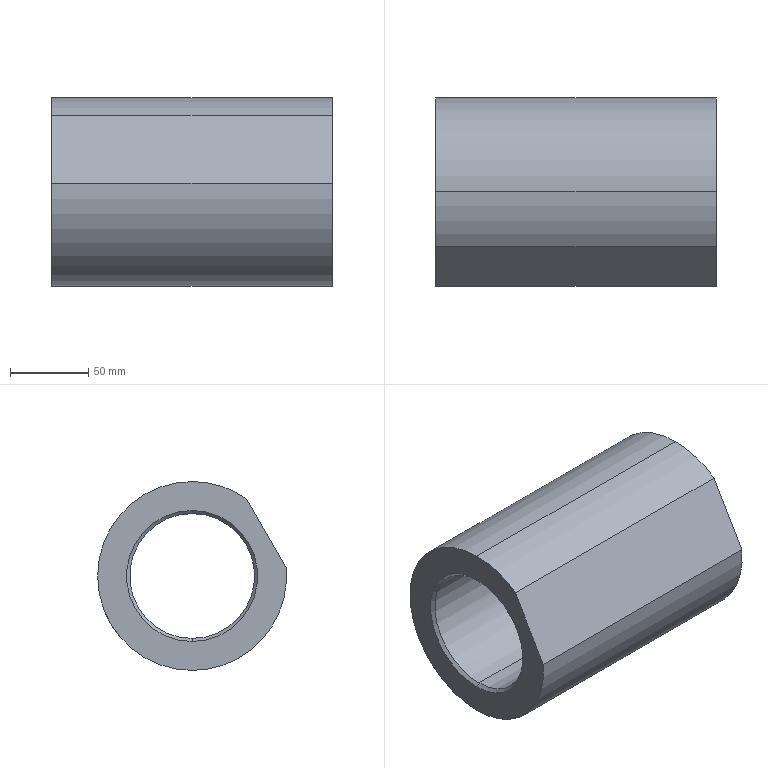Part | SolidWorks | features HoleWzd 2, Chamfer 1, Extrusion 1, ICE 1 | 1 solid | 30 faces | box 180 x 121 x 121 mm | volume 1121817 mm3 | cylinder 15 | cone 12 | plane 3 | commonest cylinder face diameters 8.5 x10 121 x3 80 x2
STEP:
#1=CARTESIAN_POINT('',(88.,0.,40.));
#2=VERTEX_POINT('',#1);
#3=CARTESIAN_POINT('',(88.,0.,-40.));
#4=VERTEX_POINT('',#3);
#5=CARTESIAN_POINT('',(88.,0.,0.));
#6=DIRECTION('',(1.,0.,0.));
#7=DIRECTION('',(0.,0.,-1.));
#8=AXIS2_PLACEMENT_3D('',#5,#6,#7);
#9=CIRCLE('',#8,40.);
#10=EDGE_CURVE('',#2,#4,#9,.T.);
#11=ORIENTED_EDGE('',*,*,#10,.F.);
#12=CARTESIAN_POINT('',(90.,0.,42.));
#13=VERTEX_POINT('',#12);
#14=CARTESIAN_POINT('',(88.,0.,40.));
#15=DIRECTION('',(0.7071,0.,0.7071));
#16=VECTOR('',#15,1000.);
#17=LINE('',#14,#16);
#18=EDGE_CURVE('',#2,#13,#17,.T.);
#19=ORIENTED_EDGE('',*,*,#18,.T.);
#20=CARTESIAN_POINT('',(90.,0.,-42.));
#21=VERTEX_POINT('',#20);
#22=CARTESIAN_POINT('',(90.,0.,0.));
#23=DIRECTION('',(-1.,0.,0.));
#24=DIRECTION('',(0.,0.,-1.));
#25=AXIS2_PLACEMENT_3D('',#22,#23,#24);
#26=CIRCLE('',#25,42.);
#27=EDGE_CURVE('',#21,#13,#26,.T.);
#28=ORIENTED_EDGE('',*,*,#27,.F.);
#29=CARTESIAN_POINT('',(88.,0.,-40.));
#30=DIRECTION('',(0.7071,0.,-0.7071));
#31=VECTOR('',#30,1000.);
#32=LINE('',#29,#31);
#33=EDGE_CURVE('',#4,#21,#32,.T.);
#34=ORIENTED_EDGE('',*,*,#33,.F.);
#35=EDGE_LOOP('',(#11,#19,#28,#34));
#36=FACE_OUTER_BOUND('',#35,.T.);
#37=CARTESIAN_POINT('',(88.,0.,0.));
#38=DIRECTION('',(1.,0.,0.));
#39=DIRECTION('',(0.,0.,-1.));
#40=AXIS2_PLACEMENT_3D('',#37,#38,#39);
#41=CONICAL_SURFACE('',#40,40.,0.7854);
#42=ADVANCED_FACE('',(#36),#41,.F.);
#43=CARTESIAN_POINT('',(-88.,0.,-40.));
#44=VERTEX_POINT('',#43);
#45=CARTESIAN_POINT('',(-88.,0.,40.));
#46=VERTEX_POINT('',#45);
#47=CARTESIAN_POINT('',(-88.,0.,0.));
#48=DIRECTION('',(-1.,0.,0.));
#49=DIRECTION('',(0.,0.,-1.));
#50=AXIS2_PLACEMENT_3D('',#47,#48,#49);
#51=CIRCLE('',#50,40.);
#52=EDGE_CURVE('',#44,#46,#51,.T.);
#53=ORIENTED_EDGE('',*,*,#52,.F.);
#54=CARTESIAN_POINT('',(-90.,0.,-42.));
#55=VERTEX_POINT('',#54);
#56=CARTESIAN_POINT('',(-90.,0.,-42.));
#57=DIRECTION('',(-0.7071,0.,-0.7071));
#58=VECTOR('',#57,1000.);
#59=LINE('',#56,#58);
#60=EDGE_CURVE('',#44,#55,#59,.T.);
#61=ORIENTED_EDGE('',*,*,#60,.T.);
#62=CARTESIAN_POINT('',(-90.,0.,42.));
#63=VERTEX_POINT('',#62);
#64=CARTESIAN_POINT('',(-90.,0.,0.));
#65=DIRECTION('',(1.,0.,0.));
#66=DIRECTION('',(0.,0.,-1.));
#67=AXIS2_PLACEMENT_3D('',#64,#65,#66);
#68=CIRCLE('',#67,42.);
#69=EDGE_CURVE('',#63,#55,#68,.T.);
#70=ORIENTED_EDGE('',*,*,#69,.F.);
#71=CARTESIAN_POINT('',(-90.,0.,42.));
#72=DIRECTION('',(-0.7071,0.,0.7071));
#73=VECTOR('',#72,1000.);
#74=LINE('',#71,#73);
#75=EDGE_CURVE('',#46,#63,#74,.T.);
#76=ORIENTED_EDGE('',*,*,#75,.F.);
#77=EDGE_LOOP('',(#53,#61,#70,#76));
#78=FACE_OUTER_BOUND('',#77,.T.);
#79=CARTESIAN_POINT('',(-90.,0.,0.));
#80=DIRECTION('',(-1.,0.,0.));
#81=DIRECTION('',(0.,0.,1.));
#82=AXIS2_PLACEMENT_3D('',#79,#80,#81);
#83=CONICAL_SURFACE('',#82,42.,0.7854);
#84=ADVANCED_FACE('',(#78),#83,.F.);
#85=CARTESIAN_POINT('',(58.,49.81,8.608));
#86=VERTEX_POINT('',#85);
#87=CARTESIAN_POINT('',(58.,49.81,0.1078));
#88=VERTEX_POINT('',#87);
#89=CARTESIAN_POINT('',(58.,49.81,4.358));
#90=DIRECTION('',(1.,0.,0.));
#91=DIRECTION('',(0.,0.,-1.));
#92=AXIS2_PLACEMENT_3D('',#89,#90,#91);
#93=CIRCLE('',#92,4.25);
#94=EDGE_CURVE('',#86,#88,#93,.T.);
#95=ORIENTED_EDGE('',*,*,#94,.F.);
#96=CARTESIAN_POINT('',(90.,49.81,8.608));
#97=VERTEX_POINT('',#96);
#98=CARTESIAN_POINT('',(90.,49.81,8.608));
#99=DIRECTION('',(1.,0.,0.));
#100=VECTOR('',#99,1000.);
#101=LINE('',#98,#100);
#102=EDGE_CURVE('',#86,#97,#101,.T.);
#103=ORIENTED_EDGE('',*,*,#102,.T.);
#104=CARTESIAN_POINT('',(90.,49.81,0.1078));
#105=VERTEX_POINT('',#104);
#106=CARTESIAN_POINT('',(90.,49.81,4.358));
#107=DIRECTION('',(1.,0.,0.));
#108=DIRECTION('',(0.,0.,-1.));
#109=AXIS2_PLACEMENT_3D('',#106,#107,#108);
#110=CIRCLE('',#109,4.25);
#111=EDGE_CURVE('',#97,#105,#110,.T.);
#112=ORIENTED_EDGE('',*,*,#111,.T.);
#113=CARTESIAN_POINT('',(90.,49.81,0.1078));
#114=DIRECTION('',(1.,0.,0.));
#115=VECTOR('',#114,1000.);
#116=LINE('',#113,#115);
#117=EDGE_CURVE('',#88,#105,#116,.T.);
#118=ORIENTED_EDGE('',*,*,#117,.F.);
#119=EDGE_LOOP('',(#95,#103,#112,#118));
#120=FACE_OUTER_BOUND('',#119,.T.);
#121=CARTESIAN_POINT('',(90.,49.81,4.358));
#122=DIRECTION('',(1.,0.,0.));
#123=DIRECTION('',(0.,0.,-1.));
#124=AXIS2_PLACEMENT_3D('',#121,#122,#123);
#125=CYLINDRICAL_SURFACE('',#124,4.25);
#126=ADVANCED_FACE('',(#120),#125,.F.);
#127=CARTESIAN_POINT('',(55.446,49.81,4.358));
#128=VERTEX_POINT('',#127);
#129=CARTESIAN_POINT('',(58.,49.81,0.1078));
#130=DIRECTION('',(0.515,0.,-0.8572));
#131=VECTOR('',#130,1000.);
#132=LINE('',#129,#131);
#133=EDGE_CURVE('',#128,#88,#132,.T.);
#134=ORIENTED_EDGE('',*,*,#133,.F.);
#135=CARTESIAN_POINT('',(58.,49.81,8.608));
#136=DIRECTION('',(0.515,0.,0.8572));
#137=VECTOR('',#136,1000.);
#138=LINE('',#135,#137);
#139=EDGE_CURVE('',#128,#86,#138,.T.);
#140=ORIENTED_EDGE('',*,*,#139,.T.);
#141=ORIENTED_EDGE('',*,*,#94,.T.);
#142=EDGE_LOOP('',(#134,#140,#141));
#143=FACE_OUTER_BOUND('',#142,.T.);
#144=CARTESIAN_POINT('',(58.,49.81,4.358));
#145=DIRECTION('',(1.,0.,0.));
#146=DIRECTION('',(0.,0.,-1.));
#147=AXIS2_PLACEMENT_3D('',#144,#145,#146);
#148=CONICAL_SURFACE('',#147,4.25,1.03);
#149=ADVANCED_FACE('',(#143),#148,.F.);
#150=CARTESIAN_POINT('',(58.,21.131,-41.065));
#151=VERTEX_POINT('',#150);
#152=CARTESIAN_POINT('',(58.,21.131,-49.565));
#153=VERTEX_POINT('',#152);
#154=CARTESIAN_POINT('',(58.,21.131,-45.315));
#155=DIRECTION('',(1.,0.,0.));
#156=DIRECTION('',(0.,0.,-1.));
#157=AXIS2_PLACEMENT_3D('',#154,#155,#156);
#158=CIRCLE('',#157,4.25);
#159=EDGE_CURVE('',#151,#153,#158,.T.);
#160=ORIENTED_EDGE('',*,*,#159,.F.);
#161=CARTESIAN_POINT('',(90.,21.131,-41.065));
#162=VERTEX_POINT('',#161);
#163=CARTESIAN_POINT('',(90.,21.131,-41.065));
#164=DIRECTION('',(1.,0.,0.));
#165=VECTOR('',#164,1000.);
#166=LINE('',#163,#165);
#167=EDGE_CURVE('',#151,#162,#166,.T.);
#168=ORIENTED_EDGE('',*,*,#167,.T.);
#169=CARTESIAN_POINT('',(90.,21.131,-49.565));
#170=VERTEX_POINT('',#169);
#171=CARTESIAN_POINT('',(90.,21.131,-45.315));
#172=DIRECTION('',(1.,0.,0.));
#173=DIRECTION('',(0.,0.,-1.));
#174=AXIS2_PLACEMENT_3D('',#171,#172,#173);
#175=CIRCLE('',#174,4.25);
#176=EDGE_CURVE('',#162,#170,#175,.T.);
#177=ORIENTED_EDGE('',*,*,#176,.T.);
#178=CARTESIAN_POINT('',(90.,21.131,-49.565));
#179=DIRECTION('',(1.,0.,0.));
#180=VECTOR('',#179,1000.);
#181=LINE('',#178,#180);
#182=EDGE_CURVE('',#153,#170,#181,.T.);
#183=ORIENTED_EDGE('',*,*,#182,.F.);
#184=EDGE_LOOP('',(#160,#168,#177,#183));
#185=FACE_OUTER_BOUND('',#184,.T.);
#186=CARTESIAN_POINT('',(90.,21.131,-45.315));
#187=DIRECTION('',(1.,0.,0.));
#188=DIRECTION('',(0.,0.,-1.));
#189=AXIS2_PLACEMENT_3D('',#186,#187,#188);
#190=CYLINDRICAL_SURFACE('',#189,4.25);
#191=ADVANCED_FACE('',(#185),#190,.F.);
#192=CARTESIAN_POINT('',(55.446,21.131,-45.315));
#193=VERTEX_POINT('',#192);
#194=CARTESIAN_POINT('',(58.,21.131,-49.565));
#195=DIRECTION('',(0.515,0.,-0.8572));
#196=VECTOR('',#195,1000.);
#197=LINE('',#194,#196);
#198=EDGE_CURVE('',#193,#153,#197,.T.);
#199=ORIENTED_EDGE('',*,*,#198,.F.);
#200=CARTESIAN_POINT('',(58.,21.131,-41.065));
#201=DIRECTION('',(0.515,0.,0.8572));
#202=VECTOR('',#201,1000.);
#203=LINE('',#200,#202);
#204=EDGE_CURVE('',#193,#151,#203,.T.);
#205=ORIENTED_EDGE('',*,*,#204,.T.);
#206=ORIENTED_EDGE('',*,*,#159,.T.);
#207=EDGE_LOOP('',(#199,#205,#206));
#208=FACE_OUTER_BOUND('',#207,.T.);
#209=CARTESIAN_POINT('',(58.,21.131,-45.315));
#210=DIRECTION('',(1.,0.,0.));
#211=DIRECTION('',(0.,0.,-1.));
#212=AXIS2_PLACEMENT_3D('',#209,#210,#211);
#213=CONICAL_SURFACE('',#212,4.25,1.03);
#214=ADVANCED_FACE('',(#208),#213,.F.);
#215=CARTESIAN_POINT('',(58.,-35.355,-31.105));
#216=VERTEX_POINT('',#215);
#217=CARTESIAN_POINT('',(58.,-35.355,-39.605));
#218=VERTEX_POINT('',#217);
#219=CARTESIAN_POINT('',(58.,-35.355,-35.355));
#220=DIRECTION('',(1.,0.,0.));
#221=DIRECTION('',(0.,0.,-1.));
#222=AXIS2_PLACEMENT_3D('',#219,#220,#221);
#223=CIRCLE('',#222,4.25);
#224=EDGE_CURVE('',#216,#218,#223,.T.);
#225=ORIENTED_EDGE('',*,*,#224,.F.);
#226=CARTESIAN_POINT('',(90.,-35.355,-31.105));
#227=VERTEX_POINT('',#226);
#228=CARTESIAN_POINT('',(90.,-35.355,-31.105));
#229=DIRECTION('',(1.,0.,0.));
#230=VECTOR('',#229,1000.);
#231=LINE('',#228,#230);
#232=EDGE_CURVE('',#216,#227,#231,.T.);
#233=ORIENTED_EDGE('',*,*,#232,.T.);
#234=CARTESIAN_POINT('',(90.,-35.355,-39.605));
#235=VERTEX_POINT('',#234);
#236=CARTESIAN_POINT('',(90.,-35.355,-35.355));
#237=DIRECTION('',(1.,0.,0.));
#238=DIRECTION('',(0.,0.,-1.));
#239=AXIS2_PLACEMENT_3D('',#236,#237,#238);
#240=CIRCLE('',#239,4.25);
#241=EDGE_CURVE('',#227,#235,#240,.T.);
#242=ORIENTED_EDGE('',*,*,#241,.T.);
#243=CARTESIAN_POINT('',(90.,-35.355,-39.605));
#244=DIRECTION('',(1.,0.,0.));
#245=VECTOR('',#244,1000.);
#246=LINE('',#243,#245);
#247=EDGE_CURVE('',#218,#235,#246,.T.);
#248=ORIENTED_EDGE('',*,*,#247,.F.);
#249=EDGE_LOOP('',(#225,#233,#242,#248));
#250=FACE_OUTER_BOUND('',#249,.T.);
#251=CARTESIAN_POINT('',(90.,-35.355,-35.355));
#252=DIRECTION('',(1.,0.,0.));
#253=DIRECTION('',(0.,0.,-1.));
#254=AXIS2_PLACEMENT_3D('',#251,#252,#253);
#255=CYLINDRICAL_SURFACE('',#254,4.25);
#256=ADVANCED_FACE('',(#250),#255,.F.);
#257=CARTESIAN_POINT('',(55.446,-35.355,-35.355));
#258=VERTEX_POINT('',#257);
#259=CARTESIAN_POINT('',(58.,-35.355,-39.605));
#260=DIRECTION('',(0.515,0.,-0.8572));
#261=VECTOR('',#260,1000.);
#262=LINE('',#259,#261);
#263=EDGE_CURVE('',#258,#218,#262,.T.);
#264=ORIENTED_EDGE('',*,*,#263,.F.);
#265=CARTESIAN_POINT('',(58.,-35.355,-31.105));
#266=DIRECTION('',(0.515,0.,0.8572));
#267=VECTOR('',#266,1000.);
#268=LINE('',#265,#267);
#269=EDGE_CURVE('',#258,#216,#268,.T.);
#270=ORIENTED_EDGE('',*,*,#269,.T.);
#271=ORIENTED_EDGE('',*,*,#224,.T.);
#272=EDGE_LOOP('',(#264,#270,#271));
#273=FACE_OUTER_BOUND('',#272,.T.);
#274=CARTESIAN_POINT('',(58.,-35.355,-35.355));
#275=DIRECTION('',(1.,0.,0.));
#276=DIRECTION('',(0.,0.,-1.));
#277=AXIS2_PLACEMENT_3D('',#274,#275,#276);
#278=CONICAL_SURFACE('',#277,4.25,1.03);
#279=ADVANCED_FACE('',(#273),#278,.F.);
#280=CARTESIAN_POINT('',(58.,12.941,52.546));
#281=VERTEX_POINT('',#280);
#282=CARTESIAN_POINT('',(58.,12.941,44.046));
#283=VERTEX_POINT('',#282);
#284=CARTESIAN_POINT('',(58.,12.941,48.296));
#285=DIRECTION('',(1.,0.,0.));
#286=DIRECTION('',(0.,0.,-1.));
#287=AXIS2_PLACEMENT_3D('',#284,#285,#286);
#288=CIRCLE('',#287,4.25);
#289=EDGE_CURVE('',#281,#283,#288,.T.);
#290=ORIENTED_EDGE('',*,*,#289,.F.);
#291=CARTESIAN_POINT('',(90.,12.941,52.546));
#292=VERTEX_POINT('',#291);
#293=CARTESIAN_POINT('',(90.,12.941,52.546));
#294=DIRECTION('',(1.,0.,0.));
#295=VECTOR('',#294,1000.);
#296=LINE('',#293,#295);
#297=EDGE_CURVE('',#281,#292,#296,.T.);
#298=ORIENTED_EDGE('',*,*,#297,.T.);
#299=CARTESIAN_POINT('',(90.,12.941,44.046));
#300=VERTEX_POINT('',#299);
#301=CARTESIAN_POINT('',(90.,12.941,48.296));
#302=DIRECTION('',(1.,0.,0.));
#303=DIRECTION('',(0.,0.,-1.));
#304=AXIS2_PLACEMENT_3D('',#301,#302,#303);
#305=CIRCLE('',#304,4.25);
#306=EDGE_CURVE('',#292,#300,#305,.T.);
#307=ORIENTED_EDGE('',*,*,#306,.T.);
#308=CARTESIAN_POINT('',(90.,12.941,44.046));
#309=DIRECTION('',(1.,0.,0.));
#310=VECTOR('',#309,1000.);
#311=LINE('',#308,#310);
#312=EDGE_CURVE('',#283,#300,#311,.T.);
#313=ORIENTED_EDGE('',*,*,#312,.F.);
#314=EDGE_LOOP('',(#290,#298,#307,#313));
#315=FACE_OUTER_BOUND('',#314,.T.);
#316=CARTESIAN_POINT('',(90.,12.941,48.296));
#317=DIRECTION('',(1.,0.,0.));
#318=DIRECTION('',(0.,0.,-1.));
#319=AXIS2_PLACEMENT_3D('',#316,#317,#318);
#320=CYLINDRICAL_SURFACE('',#319,4.25);
#321=ADVANCED_FACE('',(#315),#320,.F.);
#322=CARTESIAN_POINT('',(55.446,12.941,48.296));
#323=VERTEX_POINT('',#322);
#324=CARTESIAN_POINT('',(58.,12.941,44.046));
#325=DIRECTION('',(0.515,0.,-0.8572));
#326=VECTOR('',#325,1000.);
#327=LINE('',#324,#326);
#328=EDGE_CURVE('',#323,#283,#327,.T.);
#329=ORIENTED_EDGE('',*,*,#328,.F.);
#330=CARTESIAN_POINT('',(58.,12.941,52.546));
#331=DIRECTION('',(0.515,0.,0.8572));
#332=VECTOR('',#331,1000.);
#333=LINE('',#330,#332);
#334=EDGE_CURVE('',#323,#281,#333,.T.);
#335=ORIENTED_EDGE('',*,*,#334,.T.);
#336=ORIENTED_EDGE('',*,*,#289,.T.);
#337=EDGE_LOOP('',(#329,#335,#336));
#338=FACE_OUTER_BOUND('',#337,.T.);
#339=CARTESIAN_POINT('',(58.,12.941,48.296));
#340=DIRECTION('',(1.,0.,0.));
#341=DIRECTION('',(0.,0.,-1.));
#342=AXIS2_PLACEMENT_3D('',#339,#340,#341);
#343=CONICAL_SURFACE('',#342,4.25,1.03);
#344=ADVANCED_FACE('',(#338),#343,.F.);
#345=CARTESIAN_POINT('',(0.,54.39,-26.495));
#346=VERTEX_POINT('',#345);
#347=CARTESIAN_POINT('',(0.,50.14,-33.856));
#348=VERTEX_POINT('',#347);
#349=CARTESIAN_POINT('',(0.,54.39,-26.495));
#350=CARTESIAN_POINT('',(-0.2774,54.39,-26.495));
#351=CARTESIAN_POINT('',(-0.5531,54.378,-26.519));
#352=CARTESIAN_POINT('',(-1.101,54.33,-26.617));
#353=CARTESIAN_POINT('',(-1.37,54.294,-26.69));
#354=CARTESIAN_POINT('',(-1.881,54.201,-26.881));
#355=CARTESIAN_POINT('',(-2.128,54.142,-26.999));
#356=CARTESIAN_POINT('',(-2.593,54.002,-27.277));
#357=CARTESIAN_POINT('',(-2.807,53.923,-27.434));
#358=CARTESIAN_POINT('',(-3.199,53.744,-27.783));
#359=CARTESIAN_POINT('',(-3.379,53.643,-27.977));
#360=CARTESIAN_POINT('',(-3.687,53.428,-28.386));
#361=CARTESIAN_POINT('',(-3.818,53.313,-28.601));
#362=CARTESIAN_POINT('',(-4.032,53.068,-29.053));
#363=CARTESIAN_POINT('',(-4.114,52.938,-29.29));
#364=CARTESIAN_POINT('',(-4.222,52.673,-29.764));
#365=CARTESIAN_POINT('',(-4.25,52.536,-30.004));
#366=CARTESIAN_POINT('',(-4.25,52.256,-30.49));
#367=CARTESIAN_POINT('',(-4.223,52.116,-30.729));
#368=CARTESIAN_POINT('',(-4.115,51.838,-31.196));
#369=CARTESIAN_POINT('',(-4.034,51.698,-31.426));
#370=CARTESIAN_POINT('',(-3.821,51.429,-31.866));
#371=CARTESIAN_POINT('',(-3.69,51.299,-32.073));
#372=CARTESIAN_POINT('',(-3.383,51.053,-32.464));
#373=CARTESIAN_POINT('',(-3.203,50.935,-32.648));
#374=CARTESIAN_POINT('',(-2.811,50.722,-32.978));
#375=CARTESIAN_POINT('',(-2.598,50.625,-33.126));
#376=CARTESIAN_POINT('',(-2.134,50.454,-33.386));
#377=CARTESIAN_POINT('',(-1.886,50.381,-33.497));
#378=CARTESIAN_POINT('',(-1.375,50.263,-33.674));
#379=CARTESIAN_POINT('',(-1.108,50.217,-33.742));
#380=CARTESIAN_POINT('',(-0.5587,50.156,-33.833));
#381=CARTESIAN_POINT('',(-0.2808,50.14,-33.856));
#382=CARTESIAN_POINT('',(0.,50.14,-33.856));
#383=B_SPLINE_CURVE_WITH_KNOTS('',3,(#349,#350,#351,#352,#353,#354,#355,#356,#357,#358,#359,#360,#361,#362,#363,#364,#365,#366,#367,#368,#369,#370,#371,#372,#373,#374,#375,#376,#377,#378,#379,#380,#381,#382),.UNSPECIFIED.,.F.,.F.,(4,2,2,2,2,2,2,2,2,2,2,2,2,2,2,2,4),(0.01329,0.01412,0.01495,0.01578,0.01661,0.01744,0.01827,0.01911,0.01994,0.02077,0.0216,0.02243,0.02326,0.02409,0.02492,0.02575,0.02658),.UNSPECIFIED.);
#384=EDGE_CURVE('',#346,#348,#383,.T.);
#385=ORIENTED_EDGE('',*,*,#384,.F.);
#386=CARTESIAN_POINT('',(0.,36.57,-16.206));
#387=VERTEX_POINT('',#386);
#388=CARTESIAN_POINT('',(0.,2.125,3.681));
#389=DIRECTION('',(0.,-0.866,0.5));
#390=VECTOR('',#389,1000.);
#391=LINE('',#388,#390);
#392=EDGE_CURVE('',#346,#387,#391,.T.);
#393=ORIENTED_EDGE('',*,*,#392,.T.);
#394=CARTESIAN_POINT('',(0.,32.32,-23.567));
#395=VERTEX_POINT('',#394);
#396=CARTESIAN_POINT('',(0.,36.57,-16.206));
#397=CARTESIAN_POINT('',(-0.2774,36.57,-16.206));
#398=CARTESIAN_POINT('',(-0.5533,36.559,-16.231));
#399=CARTESIAN_POINT('',(-1.102,36.514,-16.331));
#400=CARTESIAN_POINT('',(-1.37,36.481,-16.406));
#401=CARTESIAN_POINT('',(-1.881,36.393,-16.6));
#402=CARTESIAN_POINT('',(-2.129,36.338,-16.72));
#403=CARTESIAN_POINT('',(-2.593,36.207,-17.003));
#404=CARTESIAN_POINT('',(-2.807,36.132,-17.162));
#405=CARTESIAN_POINT('',(-3.199,35.962,-17.516));
#406=CARTESIAN_POINT('',(-3.379,35.865,-17.713));
#407=CARTESIAN_POINT('',(-3.687,35.658,-18.126));
#408=CARTESIAN_POINT('',(-3.818,35.547,-18.343));
#409=CARTESIAN_POINT('',(-4.032,35.308,-18.799));
#410=CARTESIAN_POINT('',(-4.114,35.18,-19.037));
#411=CARTESIAN_POINT('',(-4.222,34.919,-19.513));
#412=CARTESIAN_POINT('',(-4.25,34.783,-19.754));
#413=CARTESIAN_POINT('',(-4.25,34.502,-20.24));
#414=CARTESIAN_POINT('',(-4.223,34.361,-20.478));
#415=CARTESIAN_POINT('',(-4.115,34.08,-20.943));
#416=CARTESIAN_POINT('',(-4.034,33.938,-21.173));
#417=CARTESIAN_POINT('',(-3.821,33.662,-21.608));
#418=CARTESIAN_POINT('',(-3.69,33.529,-21.814));
#419=CARTESIAN_POINT('',(-3.382,33.275,-22.2));
#420=CARTESIAN_POINT('',(-3.203,33.152,-22.382));
#421=CARTESIAN_POINT('',(-2.812,32.931,-22.707));
#422=CARTESIAN_POINT('',(-2.598,32.83,-22.852));
#423=CARTESIAN_POINT('',(-2.134,32.651,-23.107));
#424=CARTESIAN_POINT('',(-1.887,32.574,-23.215));
#425=CARTESIAN_POINT('',(-1.376,32.449,-23.389));
#426=CARTESIAN_POINT('',(-1.108,32.401,-23.456));
#427=CARTESIAN_POINT('',(-0.5588,32.336,-23.545));
#428=CARTESIAN_POINT('',(-0.281,32.32,-23.567));
#429=CARTESIAN_POINT('',(0.,32.32,-23.567));
#430=B_SPLINE_CURVE_WITH_KNOTS('',3,(#396,#397,#398,#399,#400,#401,#402,#403,#404,#405,#406,#407,#408,#409,#410,#411,#412,#413,#414,#415,#416,#417,#418,#419,#420,#421,#422,#423,#424,#425,#426,#427,#428,#429),.UNSPECIFIED.,.F.,.F.,(4,2,2,2,2,2,2,2,2,2,2,2,2,2,2,2,4),(0.0133,0.01413,0.01496,0.01579,0.01662,0.01745,0.01828,0.01911,0.01994,0.02077,0.02161,0.02244,0.02327,0.0241,0.02493,0.02576,0.02659),.UNSPECIFIED.);
#431=EDGE_CURVE('',#387,#395,#430,.T.);
#432=ORIENTED_EDGE('',*,*,#431,.T.);
#433=CARTESIAN_POINT('',(0.,-2.125,-3.681));
#434=DIRECTION('',(0.,-0.866,0.5));
#435=VECTOR('',#434,1000.);
#436=LINE('',#433,#435);
#437=EDGE_CURVE('',#348,#395,#436,.T.);
#438=ORIENTED_EDGE('',*,*,#437,.F.);
#439=EDGE_LOOP('',(#385,#393,#432,#438));
#440=FACE_OUTER_BOUND('',#439,.T.);
#441=CARTESIAN_POINT('',(0.,0.,0.));
#442=DIRECTION('',(0.,-0.866,0.5));
#443=DIRECTION('',(0.,-0.5,-0.866));
#444=AXIS2_PLACEMENT_3D('',#441,#442,#443);
#445=CYLINDRICAL_SURFACE('',#444,4.25);
#446=ADVANCED_FACE('',(#440),#445,.F.);
#447=ORIENTED_EDGE('',*,*,#10,.T.);
#448=CARTESIAN_POINT('',(90.,0.,-40.));
#449=DIRECTION('',(-1.,0.,0.));
#450=VECTOR('',#449,1000.);
#451=LINE('',#448,#450);
#452=EDGE_CURVE('',#4,#44,#451,.T.);
#453=ORIENTED_EDGE('',*,*,#452,.T.);
#454=ORIENTED_EDGE('',*,*,#52,.T.);
#455=CARTESIAN_POINT('',(90.,0.,40.));
#456=DIRECTION('',(-1.,0.,0.));
#457=VECTOR('',#456,1000.);
#458=LINE('',#455,#457);
#459=EDGE_CURVE('',#2,#46,#458,.T.);
#460=ORIENTED_EDGE('',*,*,#459,.F.);
#461=EDGE_LOOP('',(#447,#453,#454,#460));
#462=FACE_OUTER_BOUND('',#461,.T.);
#463=CARTESIAN_POINT('',(90.,0.,0.));
#464=DIRECTION('',(-1.,0.,0.));
#465=DIRECTION('',(0.,0.,1.));
#466=AXIS2_PLACEMENT_3D('',#463,#464,#465);
#467=CYLINDRICAL_SURFACE('',#466,40.);
#468=ADVANCED_FACE('',(#462),#467,.F.);
#469=CARTESIAN_POINT('',(0.,50.14,-33.856));
#470=CARTESIAN_POINT('',(0.2809,50.14,-33.856));
#471=CARTESIAN_POINT('',(0.5571,50.156,-33.833));
#472=CARTESIAN_POINT('',(1.1,50.216,-33.743));
#473=CARTESIAN_POINT('',(1.37,50.262,-33.675));
#474=CARTESIAN_POINT('',(1.885,50.381,-33.497));
#475=CARTESIAN_POINT('',(2.129,50.453,-33.388));
#476=CARTESIAN_POINT('',(2.591,50.623,-33.13));
#477=CARTESIAN_POINT('',(2.81,50.721,-32.98));
#478=CARTESIAN_POINT('',(3.202,50.934,-32.65));
#479=CARTESIAN_POINT('',(3.378,51.049,-32.469));
#480=CARTESIAN_POINT('',(3.688,51.297,-32.076));
#481=CARTESIAN_POINT('',(3.82,51.428,-31.866));
#482=CARTESIAN_POINT('',(4.032,51.696,-31.43));
#483=CARTESIAN_POINT('',(4.114,51.835,-31.201));
#484=CARTESIAN_POINT('',(4.223,52.116,-30.729));
#485=CARTESIAN_POINT('',(4.25,52.255,-30.491));
#486=CARTESIAN_POINT('',(4.25,52.532,-30.011));
#487=CARTESIAN_POINT('',(4.222,52.672,-29.766));
#488=CARTESIAN_POINT('',(4.114,52.938,-29.29));
#489=CARTESIAN_POINT('',(4.034,53.065,-29.058));
#490=CARTESIAN_POINT('',(3.821,53.311,-28.606));
#491=CARTESIAN_POINT('',(3.688,53.428,-28.386));
#492=CARTESIAN_POINT('',(3.38,53.643,-27.978));
#493=CARTESIAN_POINT('',(3.204,53.742,-27.787));
#494=CARTESIAN_POINT('',(2.807,53.923,-27.434));
#495=CARTESIAN_POINT('',(2.593,54.002,-27.277));
#496=CARTESIAN_POINT('',(2.132,54.141,-27.001));
#497=CARTESIAN_POINT('',(1.884,54.2,-26.882));
#498=CARTESIAN_POINT('',(1.369,54.295,-26.69));
#499=CARTESIAN_POINT('',(1.104,54.33,-26.618));
#500=CARTESIAN_POINT('',(0.5592,54.378,-26.52));
#501=CARTESIAN_POINT('',(0.2774,54.39,-26.495));
#502=CARTESIAN_POINT('',(0.,54.39,-26.495));
#503=B_SPLINE_CURVE_WITH_KNOTS('',3,(#469,#470,#471,#472,#473,#474,#475,#476,#477,#478,#479,#480,#481,#482,#483,#484,#485,#486,#487,#488,#489,#490,#491,#492,#493,#494,#495,#496,#497,#498,#499,#500,#501,#502),.UNSPECIFIED.,.F.,.F.,(4,2,2,2,2,2,2,2,2,2,2,2,2,2,2,2,4),(0.,0.0008307,0.001661,0.002492,0.003323,0.004154,0.004984,0.005815,0.006646,0.007476,0.008307,0.009138,0.009969,0.0108,0.01163,0.01246,0.01329),.UNSPECIFIED.);
#504=EDGE_CURVE('',#348,#346,#503,.T.);
#505=ORIENTED_EDGE('',*,*,#504,.T.);
#506=ORIENTED_EDGE('',*,*,#384,.T.);
#507=EDGE_LOOP('',(#505,#506));
#508=FACE_BOUND('',#507,.T.);
#509=CARTESIAN_POINT('',(90.,0.,-60.5));
#510=VERTEX_POINT('',#509);
#511=CARTESIAN_POINT('',(90.,0.,60.5));
#512=VERTEX_POINT('',#511);
#513=CARTESIAN_POINT('',(90.,0.,0.));
#514=DIRECTION('',(1.,0.,0.));
#515=DIRECTION('',(0.,0.,-1.));
#516=AXIS2_PLACEMENT_3D('',#513,#514,#515);
#517=CIRCLE('',#516,60.5);
#518=EDGE_CURVE('',#510,#512,#517,.T.);
#519=ORIENTED_EDGE('',*,*,#518,.F.);
#520=CARTESIAN_POINT('',(-90.,0.,-60.5));
#521=VERTEX_POINT('',#520);
#522=CARTESIAN_POINT('',(90.,0.,-60.5));
#523=DIRECTION('',(-1.,0.,0.));
#524=VECTOR('',#523,1000.);
#525=LINE('',#522,#524);
#526=EDGE_CURVE('',#510,#521,#525,.T.);
#527=ORIENTED_EDGE('',*,*,#526,.T.);
#528=CARTESIAN_POINT('',(-90.,0.,60.5));
#529=VERTEX_POINT('',#528);
#530=CARTESIAN_POINT('',(-90.,0.,0.));
#531=DIRECTION('',(1.,0.,0.));
#532=DIRECTION('',(0.,0.,-1.));
#533=AXIS2_PLACEMENT_3D('',#530,#531,#532);
#534=CIRCLE('',#533,60.5);
#535=EDGE_CURVE('',#521,#529,#534,.T.);
#536=ORIENTED_EDGE('',*,*,#535,.T.);
#537=CARTESIAN_POINT('',(90.,0.,60.5));
#538=DIRECTION('',(-1.,0.,0.));
#539=VECTOR('',#538,1000.);
#540=LINE('',#537,#539);
#541=EDGE_CURVE('',#512,#529,#540,.T.);
#542=ORIENTED_EDGE('',*,*,#541,.F.);
#543=EDGE_LOOP('',(#519,#527,#536,#542));
#544=FACE_OUTER_BOUND('',#543,.T.);
#545=CARTESIAN_POINT('',(90.,0.,0.));
#546=DIRECTION('',(-1.,0.,0.));
#547=DIRECTION('',(0.,0.,1.));
#548=AXIS2_PLACEMENT_3D('',#545,#546,#547);
#549=CYLINDRICAL_SURFACE('',#548,60.5);
#550=ADVANCED_FACE('',(#508,#544),#549,.T.);
#551=CARTESIAN_POINT('',(90.,-35.029,49.327));
#552=VERTEX_POINT('',#551);
#553=CARTESIAN_POINT('',(90.,0.,0.));
#554=DIRECTION('',(1.,0.,0.));
#555=DIRECTION('',(0.,0.,-1.));
#556=AXIS2_PLACEMENT_3D('',#553,#554,#555);
#557=CIRCLE('',#556,60.5);
#558=EDGE_CURVE('',#512,#552,#557,.T.);
#559=ORIENTED_EDGE('',*,*,#558,.F.);
#560=ORIENTED_EDGE('',*,*,#541,.T.);
#561=CARTESIAN_POINT('',(-90.,-35.029,49.327));
#562=VERTEX_POINT('',#561);
#563=CARTESIAN_POINT('',(-90.,0.,0.));
#564=DIRECTION('',(1.,0.,0.));
#565=DIRECTION('',(0.,0.,-1.));
#566=AXIS2_PLACEMENT_3D('',#563,#564,#565);
#567=CIRCLE('',#566,60.5);
#568=EDGE_CURVE('',#529,#562,#567,.T.);
#569=ORIENTED_EDGE('',*,*,#568,.T.);
#570=CARTESIAN_POINT('',(-90.,-35.029,49.327));
#571=DIRECTION('',(1.,0.,0.));
#572=VECTOR('',#571,1000.);
#573=LINE('',#570,#572);
#574=EDGE_CURVE('',#562,#552,#573,.T.);
#575=ORIENTED_EDGE('',*,*,#574,.T.);
#576=EDGE_LOOP('',(#559,#560,#569,#575));
#577=FACE_OUTER_BOUND('',#576,.T.);
#578=CARTESIAN_POINT('',(90.,0.,0.));
#579=DIRECTION('',(-1.,0.,0.));
#580=DIRECTION('',(0.,0.,1.));
#581=AXIS2_PLACEMENT_3D('',#578,#579,#580);
#582=CYLINDRICAL_SURFACE('',#581,60.5);
#583=ADVANCED_FACE('',(#577),#582,.T.);
#584=ORIENTED_EDGE('',*,*,#27,.T.);
#585=CARTESIAN_POINT('',(90.,0.,0.));
#586=DIRECTION('',(-1.,0.,0.));
#587=DIRECTION('',(0.,0.,-1.));
#588=AXIS2_PLACEMENT_3D('',#585,#586,#587);
#589=CIRCLE('',#588,42.);
#590=EDGE_CURVE('',#13,#21,#589,.T.);
#591=ORIENTED_EDGE('',*,*,#590,.T.);
#592=EDGE_LOOP('',(#584,#591));
#593=FACE_BOUND('',#592,.T.);
#594=CARTESIAN_POINT('',(90.,49.81,4.358));
#595=DIRECTION('',(1.,0.,0.));
#596=DIRECTION('',(0.,0.,-1.));
#597=AXIS2_PLACEMENT_3D('',#594,#595,#596);
#598=CIRCLE('',#597,4.25);
#599=EDGE_CURVE('',#105,#97,#598,.T.);
#600=ORIENTED_EDGE('',*,*,#599,.F.);
#601=ORIENTED_EDGE('',*,*,#111,.F.);
#602=EDGE_LOOP('',(#600,#601));
#603=FACE_BOUND('',#602,.T.);
#604=CARTESIAN_POINT('',(90.,21.131,-45.315));
#605=DIRECTION('',(1.,0.,0.));
#606=DIRECTION('',(0.,0.,-1.));
#607=AXIS2_PLACEMENT_3D('',#604,#605,#606);
#608=CIRCLE('',#607,4.25);
#609=EDGE_CURVE('',#170,#162,#608,.T.);
#610=ORIENTED_EDGE('',*,*,#609,.F.);
#611=ORIENTED_EDGE('',*,*,#176,.F.);
#612=EDGE_LOOP('',(#610,#611));
#613=FACE_BOUND('',#612,.T.);
#614=CARTESIAN_POINT('',(90.,-35.355,-35.355));
#615=DIRECTION('',(1.,0.,0.));
#616=DIRECTION('',(0.,0.,-1.));
#617=AXIS2_PLACEMENT_3D('',#614,#615,#616);
#618=CIRCLE('',#617,4.25);
#619=EDGE_CURVE('',#235,#227,#618,.T.);
#620=ORIENTED_EDGE('',*,*,#619,.F.);
#621=ORIENTED_EDGE('',*,*,#241,.F.);
#622=EDGE_LOOP('',(#620,#621));
#623=FACE_BOUND('',#622,.T.);
#624=CARTESIAN_POINT('',(90.,12.941,48.296));
#625=DIRECTION('',(1.,0.,0.));
#626=DIRECTION('',(0.,0.,-1.));
#627=AXIS2_PLACEMENT_3D('',#624,#625,#626);
#628=CIRCLE('',#627,4.25);
#629=EDGE_CURVE('',#300,#292,#628,.T.);
#630=ORIENTED_EDGE('',*,*,#629,.F.);
#631=ORIENTED_EDGE('',*,*,#306,.F.);
#632=EDGE_LOOP('',(#630,#631));
#633=FACE_BOUND('',#632,.T.);
#634=CARTESIAN_POINT('',(90.,-60.233,5.673));
#635=VERTEX_POINT('',#634);
#636=CARTESIAN_POINT('',(90.,-35.029,49.327));
#637=DIRECTION('',(0.,0.5,0.866));
#638=VECTOR('',#637,1000.);
#639=LINE('',#636,#638);
#640=EDGE_CURVE('',#635,#552,#639,.T.);
#641=ORIENTED_EDGE('',*,*,#640,.F.);
#642=CARTESIAN_POINT('',(90.,0.,0.));
#643=DIRECTION('',(1.,0.,0.));
#644=DIRECTION('',(0.,0.,-1.));
#645=AXIS2_PLACEMENT_3D('',#642,#643,#644);
#646=CIRCLE('',#645,60.5);
#647=EDGE_CURVE('',#635,#510,#646,.T.);
#648=ORIENTED_EDGE('',*,*,#647,.T.);
#649=ORIENTED_EDGE('',*,*,#518,.T.);
#650=ORIENTED_EDGE('',*,*,#558,.T.);
#651=EDGE_LOOP('',(#641,#648,#649,#650));
#652=FACE_OUTER_BOUND('',#651,.T.);
#653=CARTESIAN_POINT('',(90.,0.,0.));
#654=DIRECTION('',(1.,0.,0.));
#655=DIRECTION('',(0.,0.,-1.));
#656=AXIS2_PLACEMENT_3D('',#653,#654,#655);
#657=PLANE('',#656);
#658=ADVANCED_FACE('',(#593,#603,#613,#623,#633,#652),#657,.T.);
#659=ORIENTED_EDGE('',*,*,#69,.T.);
#660=CARTESIAN_POINT('',(-90.,0.,0.));
#661=DIRECTION('',(1.,0.,0.));
#662=DIRECTION('',(0.,0.,-1.));
#663=AXIS2_PLACEMENT_3D('',#660,#661,#662);
#664=CIRCLE('',#663,42.);
#665=EDGE_CURVE('',#55,#63,#664,.T.);
#666=ORIENTED_EDGE('',*,*,#665,.T.);
#667=EDGE_LOOP('',(#659,#666));
#668=FACE_BOUND('',#667,.T.);
#669=CARTESIAN_POINT('',(-90.,-60.233,5.673));
#670=VERTEX_POINT('',#669);
#671=CARTESIAN_POINT('',(-90.,0.,0.));
#672=DIRECTION('',(1.,0.,0.));
#673=DIRECTION('',(0.,0.,-1.));
#674=AXIS2_PLACEMENT_3D('',#671,#672,#673);
#675=CIRCLE('',#674,60.5);
#676=EDGE_CURVE('',#670,#521,#675,.T.);
#677=ORIENTED_EDGE('',*,*,#676,.F.);
#678=CARTESIAN_POINT('',(-90.,-35.029,49.327));
#679=DIRECTION('',(0.,0.5,0.866));
#680=VECTOR('',#679,1000.);
#681=LINE('',#678,#680);
#682=EDGE_CURVE('',#670,#562,#681,.T.);
#683=ORIENTED_EDGE('',*,*,#682,.T.);
#684=ORIENTED_EDGE('',*,*,#568,.F.);
#685=ORIENTED_EDGE('',*,*,#535,.F.);
#686=EDGE_LOOP('',(#677,#683,#684,#685));
#687=FACE_OUTER_BOUND('',#686,.T.);
#688=CARTESIAN_POINT('',(-90.,0.,0.));
#689=DIRECTION('',(1.,0.,0.));
#690=DIRECTION('',(0.,0.,-1.));
#691=AXIS2_PLACEMENT_3D('',#688,#689,#690);
#692=PLANE('',#691);
#693=ADVANCED_FACE('',(#668,#687),#692,.F.);
#694=ORIENTED_EDGE('',*,*,#526,.F.);
#695=ORIENTED_EDGE('',*,*,#647,.F.);
#696=CARTESIAN_POINT('',(-90.,-60.233,5.673));
#697=DIRECTION('',(1.,0.,0.));
#698=VECTOR('',#697,1000.);
#699=LINE('',#696,#698);
#700=EDGE_CURVE('',#670,#635,#699,.T.);
#701=ORIENTED_EDGE('',*,*,#700,.F.);
#702=ORIENTED_EDGE('',*,*,#676,.T.);
#703=EDGE_LOOP('',(#694,#695,#701,#702));
#704=FACE_OUTER_BOUND('',#703,.T.);
#705=CARTESIAN_POINT('',(90.,0.,0.));
#706=DIRECTION('',(-1.,0.,0.));
#707=DIRECTION('',(0.,0.,1.));
#708=AXIS2_PLACEMENT_3D('',#705,#706,#707);
#709=CYLINDRICAL_SURFACE('',#708,60.5);
#710=ADVANCED_FACE('',(#704),#709,.T.);
#711=ORIENTED_EDGE('',*,*,#452,.F.);
#712=CARTESIAN_POINT('',(88.,0.,0.));
#713=DIRECTION('',(1.,0.,0.));
#714=DIRECTION('',(0.,0.,-1.));
#715=AXIS2_PLACEMENT_3D('',#712,#713,#714);
#716=CIRCLE('',#715,40.);
#717=EDGE_CURVE('',#4,#2,#716,.T.);
#718=ORIENTED_EDGE('',*,*,#717,.T.);
#719=ORIENTED_EDGE('',*,*,#459,.T.);
#720=CARTESIAN_POINT('',(-88.,0.,0.));
#721=DIRECTION('',(-1.,0.,0.));
#722=DIRECTION('',(0.,0.,-1.));
#723=AXIS2_PLACEMENT_3D('',#720,#721,#722);
#724=CIRCLE('',#723,40.);
#725=EDGE_CURVE('',#46,#44,#724,.T.);
#726=ORIENTED_EDGE('',*,*,#725,.T.);
#727=EDGE_LOOP('',(#711,#718,#719,#726));
#728=FACE_OUTER_BOUND('',#727,.T.);
#729=CARTESIAN_POINT('',(0.,32.32,-23.567));
#730=CARTESIAN_POINT('',(0.281,32.32,-23.567));
#731=CARTESIAN_POINT('',(0.5573,32.336,-23.545));
#732=CARTESIAN_POINT('',(1.101,32.4,-23.457));
#733=CARTESIAN_POINT('',(1.371,32.448,-23.39));
#734=CARTESIAN_POINT('',(1.885,32.573,-23.216));
#735=CARTESIAN_POINT('',(2.13,32.649,-23.109));
#736=CARTESIAN_POINT('',(2.591,32.827,-22.856));
#737=CARTESIAN_POINT('',(2.81,32.93,-22.708));
#738=CARTESIAN_POINT('',(3.202,33.152,-22.383));
#739=CARTESIAN_POINT('',(3.378,33.271,-22.205));
#740=CARTESIAN_POINT('',(3.688,33.527,-21.817));
#741=CARTESIAN_POINT('',(3.82,33.662,-21.609));
#742=CARTESIAN_POINT('',(4.032,33.935,-21.177));
#743=CARTESIAN_POINT('',(4.114,34.077,-20.949));
#744=CARTESIAN_POINT('',(4.223,34.361,-20.479));
#745=CARTESIAN_POINT('',(4.25,34.502,-20.242));
#746=CARTESIAN_POINT('',(4.25,34.779,-19.761));
#747=CARTESIAN_POINT('',(4.222,34.917,-19.516));
#748=CARTESIAN_POINT('',(4.114,35.18,-19.038));
#749=CARTESIAN_POINT('',(4.033,35.305,-18.804));
#750=CARTESIAN_POINT('',(3.82,35.545,-18.348));
#751=CARTESIAN_POINT('',(3.687,35.658,-18.126));
#752=CARTESIAN_POINT('',(3.38,35.865,-17.714));
#753=CARTESIAN_POINT('',(3.204,35.959,-17.521));
#754=CARTESIAN_POINT('',(2.807,36.132,-17.162));
#755=CARTESIAN_POINT('',(2.593,36.207,-17.002));
#756=CARTESIAN_POINT('',(2.133,36.337,-16.722));
#757=CARTESIAN_POINT('',(1.884,36.393,-16.601));
#758=CARTESIAN_POINT('',(1.369,36.481,-16.405));
#759=CARTESIAN_POINT('',(1.104,36.514,-16.332));
#760=CARTESIAN_POINT('',(0.5593,36.559,-16.232));
#761=CARTESIAN_POINT('',(0.2775,36.57,-16.206));
#762=CARTESIAN_POINT('',(0.,36.57,-16.206));
#763=B_SPLINE_CURVE_WITH_KNOTS('',3,(#729,#730,#731,#732,#733,#734,#735,#736,#737,#738,#739,#740,#741,#742,#743,#744,#745,#746,#747,#748,#749,#750,#751,#752,#753,#754,#755,#756,#757,#758,#759,#760,#761,#762),.UNSPECIFIED.,.F.,.F.,(4,2,2,2,2,2,2,2,2,2,2,2,2,2,2,2,4),(0.,0.0008311,0.001662,0.002493,0.003324,0.004155,0.004986,0.005817,0.006648,0.007479,0.008311,0.009142,0.009973,0.0108,0.01163,0.01247,0.0133),.UNSPECIFIED.);
#764=EDGE_CURVE('',#395,#387,#763,.T.);
#765=ORIENTED_EDGE('',*,*,#764,.F.);
#766=ORIENTED_EDGE('',*,*,#431,.F.);
#767=EDGE_LOOP('',(#765,#766));
#768=FACE_BOUND('',#767,.T.);
#769=CARTESIAN_POINT('',(90.,0.,0.));
#770=DIRECTION('',(-1.,0.,0.));
#771=DIRECTION('',(0.,0.,1.));
#772=AXIS2_PLACEMENT_3D('',#769,#770,#771);
#773=CYLINDRICAL_SURFACE('',#772,40.);
#774=ADVANCED_FACE('',(#728,#768),#773,.F.);
#775=ORIENTED_EDGE('',*,*,#574,.F.);
#776=ORIENTED_EDGE('',*,*,#682,.F.);
#777=ORIENTED_EDGE('',*,*,#700,.T.);
#778=ORIENTED_EDGE('',*,*,#640,.T.);
#779=EDGE_LOOP('',(#775,#776,#777,#778));
#780=FACE_OUTER_BOUND('',#779,.T.);
#781=CARTESIAN_POINT('',(-90.,-35.029,49.327));
#782=DIRECTION('',(0.,0.866,-0.5));
#783=DIRECTION('',(0.,0.5,0.866));
#784=AXIS2_PLACEMENT_3D('',#781,#782,#783);
#785=PLANE('',#784);
#786=ADVANCED_FACE('',(#780),#785,.F.);
#787=ORIENTED_EDGE('',*,*,#392,.F.);
#788=ORIENTED_EDGE('',*,*,#504,.F.);
#789=ORIENTED_EDGE('',*,*,#437,.T.);
#790=ORIENTED_EDGE('',*,*,#764,.T.);
#791=EDGE_LOOP('',(#787,#788,#789,#790));
#792=FACE_OUTER_BOUND('',#791,.T.);
#793=CARTESIAN_POINT('',(0.,0.,0.));
#794=DIRECTION('',(0.,-0.866,0.5));
#795=DIRECTION('',(0.,-0.5,-0.866));
#796=AXIS2_PLACEMENT_3D('',#793,#794,#795);
#797=CYLINDRICAL_SURFACE('',#796,4.25);
#798=ADVANCED_FACE('',(#792),#797,.F.);
#799=ORIENTED_EDGE('',*,*,#334,.F.);
#800=ORIENTED_EDGE('',*,*,#328,.T.);
#801=CARTESIAN_POINT('',(58.,12.941,48.296));
#802=DIRECTION('',(1.,0.,0.));
#803=DIRECTION('',(0.,0.,-1.));
#804=AXIS2_PLACEMENT_3D('',#801,#802,#803);
#805=CIRCLE('',#804,4.25);
#806=EDGE_CURVE('',#283,#281,#805,.T.);
#807=ORIENTED_EDGE('',*,*,#806,.T.);
#808=EDGE_LOOP('',(#799,#800,#807));
#809=FACE_OUTER_BOUND('',#808,.T.);
#810=CARTESIAN_POINT('',(58.,12.941,48.296));
#811=DIRECTION('',(1.,0.,0.));
#812=DIRECTION('',(0.,0.,-1.));
#813=AXIS2_PLACEMENT_3D('',#810,#811,#812);
#814=CONICAL_SURFACE('',#813,4.25,1.03);
#815=ADVANCED_FACE('',(#809),#814,.F.);
#816=ORIENTED_EDGE('',*,*,#297,.F.);
#817=ORIENTED_EDGE('',*,*,#806,.F.);
#818=ORIENTED_EDGE('',*,*,#312,.T.);
#819=ORIENTED_EDGE('',*,*,#629,.T.);
#820=EDGE_LOOP('',(#816,#817,#818,#819));
#821=FACE_OUTER_BOUND('',#820,.T.);
#822=CARTESIAN_POINT('',(90.,12.941,48.296));
#823=DIRECTION('',(1.,0.,0.));
#824=DIRECTION('',(0.,0.,-1.));
#825=AXIS2_PLACEMENT_3D('',#822,#823,#824);
#826=CYLINDRICAL_SURFACE('',#825,4.25);
#827=ADVANCED_FACE('',(#821),#826,.F.);
#828=ORIENTED_EDGE('',*,*,#269,.F.);
#829=ORIENTED_EDGE('',*,*,#263,.T.);
#830=CARTESIAN_POINT('',(58.,-35.355,-35.355));
#831=DIRECTION('',(1.,0.,0.));
#832=DIRECTION('',(0.,0.,-1.));
#833=AXIS2_PLACEMENT_3D('',#830,#831,#832);
#834=CIRCLE('',#833,4.25);
#835=EDGE_CURVE('',#218,#216,#834,.T.);
#836=ORIENTED_EDGE('',*,*,#835,.T.);
#837=EDGE_LOOP('',(#828,#829,#836));
#838=FACE_OUTER_BOUND('',#837,.T.);
#839=CARTESIAN_POINT('',(58.,-35.355,-35.355));
#840=DIRECTION('',(1.,0.,0.));
#841=DIRECTION('',(0.,0.,-1.));
#842=AXIS2_PLACEMENT_3D('',#839,#840,#841);
#843=CONICAL_SURFACE('',#842,4.25,1.03);
#844=ADVANCED_FACE('',(#838),#843,.F.);
#845=ORIENTED_EDGE('',*,*,#232,.F.);
#846=ORIENTED_EDGE('',*,*,#835,.F.);
#847=ORIENTED_EDGE('',*,*,#247,.T.);
#848=ORIENTED_EDGE('',*,*,#619,.T.);
#849=EDGE_LOOP('',(#845,#846,#847,#848));
#850=FACE_OUTER_BOUND('',#849,.T.);
#851=CARTESIAN_POINT('',(90.,-35.355,-35.355));
#852=DIRECTION('',(1.,0.,0.));
#853=DIRECTION('',(0.,0.,-1.));
#854=AXIS2_PLACEMENT_3D('',#851,#852,#853);
#855=CYLINDRICAL_SURFACE('',#854,4.25);
#856=ADVANCED_FACE('',(#850),#855,.F.);
#857=ORIENTED_EDGE('',*,*,#204,.F.);
#858=ORIENTED_EDGE('',*,*,#198,.T.);
#859=CARTESIAN_POINT('',(58.,21.131,-45.315));
#860=DIRECTION('',(1.,0.,0.));
#861=DIRECTION('',(0.,0.,-1.));
#862=AXIS2_PLACEMENT_3D('',#859,#860,#861);
#863=CIRCLE('',#862,4.25);
#864=EDGE_CURVE('',#153,#151,#863,.T.);
#865=ORIENTED_EDGE('',*,*,#864,.T.);
#866=EDGE_LOOP('',(#857,#858,#865));
#867=FACE_OUTER_BOUND('',#866,.T.);
#868=CARTESIAN_POINT('',(58.,21.131,-45.315));
#869=DIRECTION('',(1.,0.,0.));
#870=DIRECTION('',(0.,0.,-1.));
#871=AXIS2_PLACEMENT_3D('',#868,#869,#870);
#872=CONICAL_SURFACE('',#871,4.25,1.03);
#873=ADVANCED_FACE('',(#867),#872,.F.);
#874=ORIENTED_EDGE('',*,*,#167,.F.);
#875=ORIENTED_EDGE('',*,*,#864,.F.);
#876=ORIENTED_EDGE('',*,*,#182,.T.);
#877=ORIENTED_EDGE('',*,*,#609,.T.);
#878=EDGE_LOOP('',(#874,#875,#876,#877));
#879=FACE_OUTER_BOUND('',#878,.T.);
#880=CARTESIAN_POINT('',(90.,21.131,-45.315));
#881=DIRECTION('',(1.,0.,0.));
#882=DIRECTION('',(0.,0.,-1.));
#883=AXIS2_PLACEMENT_3D('',#880,#881,#882);
#884=CYLINDRICAL_SURFACE('',#883,4.25);
#885=ADVANCED_FACE('',(#879),#884,.F.);
#886=ORIENTED_EDGE('',*,*,#139,.F.);
#887=ORIENTED_EDGE('',*,*,#133,.T.);
#888=CARTESIAN_POINT('',(58.,49.81,4.358));
#889=DIRECTION('',(1.,0.,0.));
#890=DIRECTION('',(0.,0.,-1.));
#891=AXIS2_PLACEMENT_3D('',#888,#889,#890);
#892=CIRCLE('',#891,4.25);
#893=EDGE_CURVE('',#88,#86,#892,.T.);
#894=ORIENTED_EDGE('',*,*,#893,.T.);
#895=EDGE_LOOP('',(#886,#887,#894));
#896=FACE_OUTER_BOUND('',#895,.T.);
#897=CARTESIAN_POINT('',(58.,49.81,4.358));
#898=DIRECTION('',(1.,0.,0.));
#899=DIRECTION('',(0.,0.,-1.));
#900=AXIS2_PLACEMENT_3D('',#897,#898,#899);
#901=CONICAL_SURFACE('',#900,4.25,1.03);
#902=ADVANCED_FACE('',(#896),#901,.F.);
#903=ORIENTED_EDGE('',*,*,#102,.F.);
#904=ORIENTED_EDGE('',*,*,#893,.F.);
#905=ORIENTED_EDGE('',*,*,#117,.T.);
#906=ORIENTED_EDGE('',*,*,#599,.T.);
#907=EDGE_LOOP('',(#903,#904,#905,#906));
#908=FACE_OUTER_BOUND('',#907,.T.);
#909=CARTESIAN_POINT('',(90.,49.81,4.358));
#910=DIRECTION('',(1.,0.,0.));
#911=DIRECTION('',(0.,0.,-1.));
#912=AXIS2_PLACEMENT_3D('',#909,#910,#911);
#913=CYLINDRICAL_SURFACE('',#912,4.25);
#914=ADVANCED_FACE('',(#908),#913,.F.);
#915=ORIENTED_EDGE('',*,*,#60,.F.);
#916=ORIENTED_EDGE('',*,*,#725,.F.);
#917=ORIENTED_EDGE('',*,*,#75,.T.);
#918=ORIENTED_EDGE('',*,*,#665,.F.);
#919=EDGE_LOOP('',(#915,#916,#917,#918));
#920=FACE_OUTER_BOUND('',#919,.T.);
#921=CARTESIAN_POINT('',(-90.,0.,0.));
#922=DIRECTION('',(-1.,0.,0.));
#923=DIRECTION('',(0.,0.,1.));
#924=AXIS2_PLACEMENT_3D('',#921,#922,#923);
#925=CONICAL_SURFACE('',#924,42.,0.7854);
#926=ADVANCED_FACE('',(#920),#925,.F.);
#927=ORIENTED_EDGE('',*,*,#18,.F.);
#928=ORIENTED_EDGE('',*,*,#717,.F.);
#929=ORIENTED_EDGE('',*,*,#33,.T.);
#930=ORIENTED_EDGE('',*,*,#590,.F.);
#931=EDGE_LOOP('',(#927,#928,#929,#930));
#932=FACE_OUTER_BOUND('',#931,.T.);
#933=CARTESIAN_POINT('',(88.,0.,0.));
#934=DIRECTION('',(1.,0.,0.));
#935=DIRECTION('',(0.,0.,-1.));
#936=AXIS2_PLACEMENT_3D('',#933,#934,#935);
#937=CONICAL_SURFACE('',#936,40.,0.7854);
#938=ADVANCED_FACE('',(#932),#937,.F.);
#939=CLOSED_SHELL('',(#42,#84,#126,#149,#191,#214,#256,#279,#321,#344,#446,#468,#550,#583,#658,#693,#710,#774,#786,#798,#815,#827,#844,#856,#873,#885,#902,#914,#926,#938));
#940=MANIFOLD_SOLID_BREP('',#939);
#941=CARTESIAN_POINT('',(0.,0.,0.));
#942=DIRECTION('',(0.,0.,1.));
#943=DIRECTION('',(1.,0.,0.));
#944=AXIS2_PLACEMENT_3D('',#941,#942,#943);
#945=(LENGTH_UNIT()NAMED_UNIT(*)SI_UNIT(.MILLI.,.METRE.));
#946=UNCERTAINTY_MEASURE_WITH_UNIT(LENGTH_MEASURE(0.00001),#945,'','');
#947=(NAMED_UNIT(*)PLANE_ANGLE_UNIT()SI_UNIT($,.RADIAN.));
#948=(NAMED_UNIT(*)SI_UNIT($,.STERADIAN.)SOLID_ANGLE_UNIT());
#949=(GEOMETRIC_REPRESENTATION_CONTEXT(3)GLOBAL_UNCERTAINTY_ASSIGNED_CONTEXT((#946))GLOBAL_UNIT_ASSIGNED_CONTEXT((#945,#947,#948))REPRESENTATION_CONTEXT('',''));
#950=ADVANCED_BREP_SHAPE_REPRESENTATION('',(#940,#944),#949);